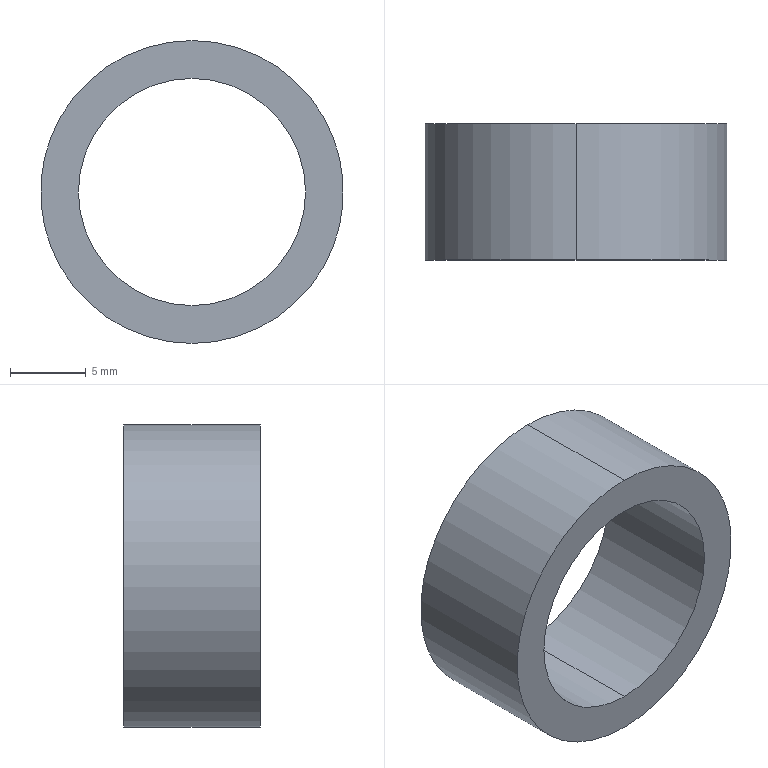Part | SolidWorks | features BaseBody 1 | 1 solid | 6 faces | box 20 x 9 x 20 mm | volume 1237 mm3 | cylinder 4 | plane 2 | commonest cylinder face diameters 15 x2 20 x2
STEP:
#1=CARTESIAN_POINT('',(0.,9.,-10.));
#2=VERTEX_POINT('',#1);
#3=CARTESIAN_POINT('',(0.,9.,10.));
#4=VERTEX_POINT('',#3);
#5=CARTESIAN_POINT('',(0.,9.,0.));
#6=DIRECTION('',(0.,-1.,0.));
#7=DIRECTION('',(0.,0.,-1.));
#8=AXIS2_PLACEMENT_3D('',#5,#6,#7);
#9=CIRCLE('',#8,10.);
#10=EDGE_CURVE('',#2,#4,#9,.T.);
#11=ORIENTED_EDGE('',*,*,#10,.T.);
#12=CARTESIAN_POINT('',(0.,0.,10.));
#13=VERTEX_POINT('',#12);
#14=CARTESIAN_POINT('',(0.,9.,10.));
#15=DIRECTION('',(0.,-1.,0.));
#16=VECTOR('',#15,1000.);
#17=LINE('',#14,#16);
#18=EDGE_CURVE('',#4,#13,#17,.T.);
#19=ORIENTED_EDGE('',*,*,#18,.T.);
#20=CARTESIAN_POINT('',(0.,0.,-10.));
#21=VERTEX_POINT('',#20);
#22=CARTESIAN_POINT('',(0.,0.,0.));
#23=DIRECTION('',(0.,1.,0.));
#24=DIRECTION('',(0.,0.,-1.));
#25=AXIS2_PLACEMENT_3D('',#22,#23,#24);
#26=CIRCLE('',#25,10.);
#27=EDGE_CURVE('',#13,#21,#26,.T.);
#28=ORIENTED_EDGE('',*,*,#27,.T.);
#29=CARTESIAN_POINT('',(0.,9.,-10.));
#30=DIRECTION('',(0.,-1.,0.));
#31=VECTOR('',#30,1000.);
#32=LINE('',#29,#31);
#33=EDGE_CURVE('',#2,#21,#32,.T.);
#34=ORIENTED_EDGE('',*,*,#33,.F.);
#35=EDGE_LOOP('',(#11,#19,#28,#34));
#36=FACE_OUTER_BOUND('',#35,.T.);
#37=CARTESIAN_POINT('',(0.,9.,0.));
#38=DIRECTION('',(0.,-1.,0.));
#39=DIRECTION('',(0.,0.,-1.));
#40=AXIS2_PLACEMENT_3D('',#37,#38,#39);
#41=CYLINDRICAL_SURFACE('',#40,10.);
#42=ADVANCED_FACE('',(#36),#41,.T.);
#43=CARTESIAN_POINT('',(0.,9.,7.5));
#44=VERTEX_POINT('',#43);
#45=CARTESIAN_POINT('',(0.,9.,-7.5));
#46=VERTEX_POINT('',#45);
#47=CARTESIAN_POINT('',(0.,9.,0.));
#48=DIRECTION('',(0.,-1.,0.));
#49=DIRECTION('',(0.,0.,-1.));
#50=AXIS2_PLACEMENT_3D('',#47,#48,#49);
#51=CIRCLE('',#50,7.5);
#52=EDGE_CURVE('',#44,#46,#51,.T.);
#53=ORIENTED_EDGE('',*,*,#52,.F.);
#54=CARTESIAN_POINT('',(0.,0.,7.5));
#55=VERTEX_POINT('',#54);
#56=CARTESIAN_POINT('',(0.,9.,7.5));
#57=DIRECTION('',(0.,-1.,0.));
#58=VECTOR('',#57,1000.);
#59=LINE('',#56,#58);
#60=EDGE_CURVE('',#44,#55,#59,.T.);
#61=ORIENTED_EDGE('',*,*,#60,.T.);
#62=CARTESIAN_POINT('',(0.,0.,-7.5));
#63=VERTEX_POINT('',#62);
#64=CARTESIAN_POINT('',(0.,0.,0.));
#65=DIRECTION('',(0.,-1.,0.));
#66=DIRECTION('',(0.,0.,-1.));
#67=AXIS2_PLACEMENT_3D('',#64,#65,#66);
#68=CIRCLE('',#67,7.5);
#69=EDGE_CURVE('',#55,#63,#68,.T.);
#70=ORIENTED_EDGE('',*,*,#69,.T.);
#71=CARTESIAN_POINT('',(0.,9.,-7.5));
#72=DIRECTION('',(0.,-1.,0.));
#73=VECTOR('',#72,1000.);
#74=LINE('',#71,#73);
#75=EDGE_CURVE('',#46,#63,#74,.T.);
#76=ORIENTED_EDGE('',*,*,#75,.F.);
#77=EDGE_LOOP('',(#53,#61,#70,#76));
#78=FACE_OUTER_BOUND('',#77,.T.);
#79=CARTESIAN_POINT('',(0.,9.,0.));
#80=DIRECTION('',(0.,-1.,0.));
#81=DIRECTION('',(0.,0.,-1.));
#82=AXIS2_PLACEMENT_3D('',#79,#80,#81);
#83=CYLINDRICAL_SURFACE('',#82,7.5);
#84=ADVANCED_FACE('',(#78),#83,.F.);
#85=ORIENTED_EDGE('',*,*,#18,.F.);
#86=CARTESIAN_POINT('',(0.,9.,0.));
#87=DIRECTION('',(0.,-1.,0.));
#88=DIRECTION('',(0.,0.,-1.));
#89=AXIS2_PLACEMENT_3D('',#86,#87,#88);
#90=CIRCLE('',#89,10.);
#91=EDGE_CURVE('',#4,#2,#90,.T.);
#92=ORIENTED_EDGE('',*,*,#91,.T.);
#93=ORIENTED_EDGE('',*,*,#33,.T.);
#94=CARTESIAN_POINT('',(0.,0.,0.));
#95=DIRECTION('',(0.,1.,0.));
#96=DIRECTION('',(0.,0.,-1.));
#97=AXIS2_PLACEMENT_3D('',#94,#95,#96);
#98=CIRCLE('',#97,10.);
#99=EDGE_CURVE('',#21,#13,#98,.T.);
#100=ORIENTED_EDGE('',*,*,#99,.T.);
#101=EDGE_LOOP('',(#85,#92,#93,#100));
#102=FACE_OUTER_BOUND('',#101,.T.);
#103=CARTESIAN_POINT('',(0.,9.,0.));
#104=DIRECTION('',(0.,-1.,0.));
#105=DIRECTION('',(0.,0.,-1.));
#106=AXIS2_PLACEMENT_3D('',#103,#104,#105);
#107=CYLINDRICAL_SURFACE('',#106,10.);
#108=ADVANCED_FACE('',(#102),#107,.T.);
#109=CARTESIAN_POINT('',(0.,0.,0.));
#110=DIRECTION('',(0.,-1.,0.));
#111=DIRECTION('',(0.,0.,-1.));
#112=AXIS2_PLACEMENT_3D('',#109,#110,#111);
#113=CIRCLE('',#112,7.5);
#114=EDGE_CURVE('',#63,#55,#113,.T.);
#115=ORIENTED_EDGE('',*,*,#114,.F.);
#116=ORIENTED_EDGE('',*,*,#69,.F.);
#117=EDGE_LOOP('',(#115,#116));
#118=FACE_BOUND('',#117,.T.);
#119=ORIENTED_EDGE('',*,*,#99,.F.);
#120=ORIENTED_EDGE('',*,*,#27,.F.);
#121=EDGE_LOOP('',(#119,#120));
#122=FACE_OUTER_BOUND('',#121,.T.);
#123=CARTESIAN_POINT('',(0.,0.,0.));
#124=DIRECTION('',(0.,1.,0.));
#125=DIRECTION('',(0.,0.,1.));
#126=AXIS2_PLACEMENT_3D('',#123,#124,#125);
#127=PLANE('',#126);
#128=ADVANCED_FACE('',(#118,#122),#127,.F.);
#129=CARTESIAN_POINT('',(0.,9.,0.));
#130=DIRECTION('',(0.,-1.,0.));
#131=DIRECTION('',(0.,0.,-1.));
#132=AXIS2_PLACEMENT_3D('',#129,#130,#131);
#133=CIRCLE('',#132,7.5);
#134=EDGE_CURVE('',#46,#44,#133,.T.);
#135=ORIENTED_EDGE('',*,*,#134,.T.);
#136=ORIENTED_EDGE('',*,*,#52,.T.);
#137=EDGE_LOOP('',(#135,#136));
#138=FACE_BOUND('',#137,.T.);
#139=ORIENTED_EDGE('',*,*,#10,.F.);
#140=ORIENTED_EDGE('',*,*,#91,.F.);
#141=EDGE_LOOP('',(#139,#140));
#142=FACE_OUTER_BOUND('',#141,.T.);
#143=CARTESIAN_POINT('',(0.,9.,0.));
#144=DIRECTION('',(0.,1.,0.));
#145=DIRECTION('',(0.,0.,1.));
#146=AXIS2_PLACEMENT_3D('',#143,#144,#145);
#147=PLANE('',#146);
#148=ADVANCED_FACE('',(#138,#142),#147,.T.);
#149=ORIENTED_EDGE('',*,*,#60,.F.);
#150=ORIENTED_EDGE('',*,*,#134,.F.);
#151=ORIENTED_EDGE('',*,*,#75,.T.);
#152=ORIENTED_EDGE('',*,*,#114,.T.);
#153=EDGE_LOOP('',(#149,#150,#151,#152));
#154=FACE_OUTER_BOUND('',#153,.T.);
#155=CARTESIAN_POINT('',(0.,9.,0.));
#156=DIRECTION('',(0.,-1.,0.));
#157=DIRECTION('',(0.,0.,-1.));
#158=AXIS2_PLACEMENT_3D('',#155,#156,#157);
#159=CYLINDRICAL_SURFACE('',#158,7.5);
#160=ADVANCED_FACE('',(#154),#159,.F.);
#161=CLOSED_SHELL('',(#42,#84,#108,#128,#148,#160));
#162=MANIFOLD_SOLID_BREP('',#161);
#163=CARTESIAN_POINT('',(0.,0.,0.));
#164=DIRECTION('',(0.,0.,1.));
#165=DIRECTION('',(1.,0.,0.));
#166=AXIS2_PLACEMENT_3D('',#163,#164,#165);
#167=(LENGTH_UNIT()NAMED_UNIT(*)SI_UNIT(.MILLI.,.METRE.));
#168=UNCERTAINTY_MEASURE_WITH_UNIT(LENGTH_MEASURE(0.00001),#167,'','');
#169=(NAMED_UNIT(*)PLANE_ANGLE_UNIT()SI_UNIT($,.RADIAN.));
#170=(NAMED_UNIT(*)SI_UNIT($,.STERADIAN.)SOLID_ANGLE_UNIT());
#171=(GEOMETRIC_REPRESENTATION_CONTEXT(3)GLOBAL_UNCERTAINTY_ASSIGNED_CONTEXT((#168))GLOBAL_UNIT_ASSIGNED_CONTEXT((#167,#169,#170))REPRESENTATION_CONTEXT('',''));
#172=ADVANCED_BREP_SHAPE_REPRESENTATION('',(#162,#166),#171);